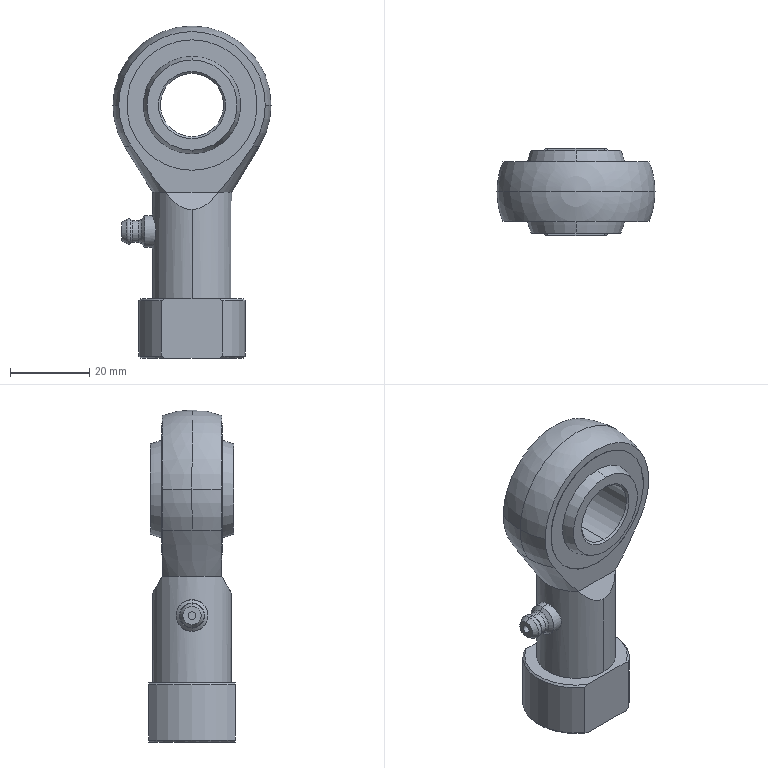Part | STEP file | F_M16150U_F-M16150U-P | 1 solid | 70 faces | box 40 x 22 x 84 mm | volume 29098 mm3 | cone 21 | cylinder 20 | plane 15 | sphere 6 | torus 4 | other 4 | commonest cylinder face diameters 33 x4 2 x2 4.917 x2 5.5 x2 8 x2 14.376 x2